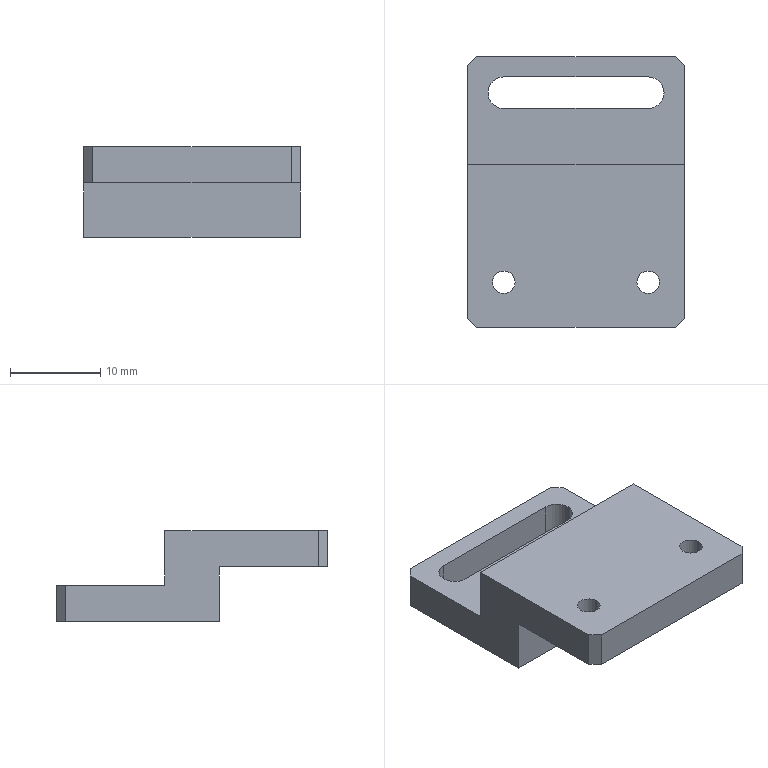Part | NX | features BREP 1 | 1 solid | 23 faces | box 24 x 30 x 10 mm | volume 3434 mm3 | plane 16 | cylinder 7 | commonest cylinder face diameters 2.5 x4 3.5 x3
STEP:
#1=CARTESIAN_POINT('',(9.25,-10.,6.));
#2=VERTEX_POINT('',#1);
#3=CARTESIAN_POINT('',(6.75,-10.,6.));
#4=VERTEX_POINT('',#3);
#5=CARTESIAN_POINT('',(8.,-10.,6.));
#6=DIRECTION('',(0.,0.,-1.));
#7=DIRECTION('',(1.,0.,0.));
#8=AXIS2_PLACEMENT_3D('',#5,#6,#7);
#9=CIRCLE('',#8,1.25);
#10=EDGE_CURVE('',#2,#4,#9,.T.);
#11=ORIENTED_EDGE('',*,*,#10,.T.);
#12=CARTESIAN_POINT('',(6.75,-10.,10.));
#13=VERTEX_POINT('',#12);
#14=CARTESIAN_POINT('',(6.75,-10.,10.));
#15=DIRECTION('',(0.,0.,1.));
#16=VECTOR('',#15,1000.);
#17=LINE('',#14,#16);
#18=EDGE_CURVE('',#13,#4,#17,.F.);
#19=ORIENTED_EDGE('',*,*,#18,.F.);
#20=CARTESIAN_POINT('',(9.25,-10.,10.));
#21=VERTEX_POINT('',#20);
#22=CARTESIAN_POINT('',(8.,-10.,10.));
#23=DIRECTION('',(0.,0.,1.));
#24=DIRECTION('',(1.,0.,0.));
#25=AXIS2_PLACEMENT_3D('',#22,#23,#24);
#26=CIRCLE('',#25,1.25);
#27=EDGE_CURVE('',#13,#21,#26,.T.);
#28=ORIENTED_EDGE('',*,*,#27,.T.);
#29=CARTESIAN_POINT('',(9.25,-10.,10.));
#30=DIRECTION('',(0.,0.,1.));
#31=VECTOR('',#30,1000.);
#32=LINE('',#29,#31);
#33=EDGE_CURVE('',#21,#2,#32,.F.);
#34=ORIENTED_EDGE('',*,*,#33,.T.);
#35=EDGE_LOOP('',(#11,#19,#28,#34));
#36=FACE_BOUND('',#35,.T.);
#37=CARTESIAN_POINT('',(8.,-10.,10.));
#38=DIRECTION('',(0.,0.,1.));
#39=DIRECTION('',(1.,0.,0.));
#40=AXIS2_PLACEMENT_3D('',#37,#38,#39);
#41=CYLINDRICAL_SURFACE('',#40,1.25);
#42=ADVANCED_FACE('',(#36),#41,.F.);
#43=CARTESIAN_POINT('',(-6.75,-10.,10.));
#44=VERTEX_POINT('',#43);
#45=CARTESIAN_POINT('',(-9.25,-10.,10.));
#46=VERTEX_POINT('',#45);
#47=CARTESIAN_POINT('',(-8.,-10.,10.));
#48=DIRECTION('',(0.,0.,-1.));
#49=DIRECTION('',(-1.,0.,0.));
#50=AXIS2_PLACEMENT_3D('',#47,#48,#49);
#51=CIRCLE('',#50,1.25);
#52=EDGE_CURVE('',#44,#46,#51,.T.);
#53=ORIENTED_EDGE('',*,*,#52,.F.);
#54=CARTESIAN_POINT('',(-6.75,-10.,6.));
#55=VERTEX_POINT('',#54);
#56=CARTESIAN_POINT('',(-6.75,-10.,0.));
#57=DIRECTION('',(0.,0.,-1.));
#58=VECTOR('',#57,1000.);
#59=LINE('',#56,#58);
#60=EDGE_CURVE('',#44,#55,#59,.T.);
#61=ORIENTED_EDGE('',*,*,#60,.T.);
#62=CARTESIAN_POINT('',(-9.25,-10.,6.));
#63=VERTEX_POINT('',#62);
#64=CARTESIAN_POINT('',(-8.,-10.,6.));
#65=DIRECTION('',(0.,0.,-1.));
#66=DIRECTION('',(1.,0.,0.));
#67=AXIS2_PLACEMENT_3D('',#64,#65,#66);
#68=CIRCLE('',#67,1.25);
#69=EDGE_CURVE('',#55,#63,#68,.T.);
#70=ORIENTED_EDGE('',*,*,#69,.T.);
#71=CARTESIAN_POINT('',(-9.25,-10.,0.));
#72=DIRECTION('',(0.,0.,-1.));
#73=VECTOR('',#72,1000.);
#74=LINE('',#71,#73);
#75=EDGE_CURVE('',#46,#63,#74,.T.);
#76=ORIENTED_EDGE('',*,*,#75,.F.);
#77=EDGE_LOOP('',(#53,#61,#70,#76));
#78=FACE_BOUND('',#77,.T.);
#79=CARTESIAN_POINT('',(-8.,-10.,0.));
#80=DIRECTION('',(0.,0.,-1.));
#81=DIRECTION('',(-1.,0.,0.));
#82=AXIS2_PLACEMENT_3D('',#79,#80,#81);
#83=CYLINDRICAL_SURFACE('',#82,1.25);
#84=ADVANCED_FACE('',(#78),#83,.F.);
#85=CARTESIAN_POINT('',(8.,12.75,0.));
#86=VERTEX_POINT('',#85);
#87=CARTESIAN_POINT('',(9.75,11.,0.));
#88=VERTEX_POINT('',#87);
#89=CARTESIAN_POINT('',(8.,11.,0.));
#90=DIRECTION('',(0.,0.,-1.));
#91=DIRECTION('',(-1.,0.,0.));
#92=AXIS2_PLACEMENT_3D('',#89,#90,#91);
#93=CIRCLE('',#92,1.75);
#94=EDGE_CURVE('',#86,#88,#93,.T.);
#95=ORIENTED_EDGE('',*,*,#94,.T.);
#96=CARTESIAN_POINT('',(9.75,11.,4.));
#97=VERTEX_POINT('',#96);
#98=CARTESIAN_POINT('',(9.75,11.,-5.));
#99=DIRECTION('',(0.,0.,1.));
#100=VECTOR('',#99,1000.);
#101=LINE('',#98,#100);
#102=EDGE_CURVE('',#88,#97,#101,.T.);
#103=ORIENTED_EDGE('',*,*,#102,.T.);
#104=CARTESIAN_POINT('',(8.,12.75,4.));
#105=VERTEX_POINT('',#104);
#106=CARTESIAN_POINT('',(8.,11.,4.));
#107=DIRECTION('',(0.,0.,1.));
#108=DIRECTION('',(-1.,0.,0.));
#109=AXIS2_PLACEMENT_3D('',#106,#107,#108);
#110=CIRCLE('',#109,1.75);
#111=EDGE_CURVE('',#97,#105,#110,.T.);
#112=ORIENTED_EDGE('',*,*,#111,.T.);
#113=CARTESIAN_POINT('',(8.,12.75,-5.));
#114=DIRECTION('',(0.,0.,1.));
#115=VECTOR('',#114,1000.);
#116=LINE('',#113,#115);
#117=EDGE_CURVE('',#86,#105,#116,.T.);
#118=ORIENTED_EDGE('',*,*,#117,.F.);
#119=EDGE_LOOP('',(#95,#103,#112,#118));
#120=FACE_BOUND('',#119,.T.);
#121=CARTESIAN_POINT('',(8.,11.,-5.));
#122=DIRECTION('',(0.,0.,1.));
#123=DIRECTION('',(1.,0.,0.));
#124=AXIS2_PLACEMENT_3D('',#121,#122,#123);
#125=CYLINDRICAL_SURFACE('',#124,1.75);
#126=ADVANCED_FACE('',(#120),#125,.F.);
#127=CARTESIAN_POINT('',(12.,-3.,0.));
#128=VERTEX_POINT('',#127);
#129=CARTESIAN_POINT('',(12.,14.,0.));
#130=VERTEX_POINT('',#129);
#131=CARTESIAN_POINT('',(12.,-15.,0.));
#132=DIRECTION('',(0.,1.,0.));
#133=VECTOR('',#132,1000.);
#134=LINE('',#131,#133);
#135=EDGE_CURVE('',#128,#130,#134,.T.);
#136=ORIENTED_EDGE('',*,*,#135,.T.);
#137=CARTESIAN_POINT('',(12.,14.,4.));
#138=VERTEX_POINT('',#137);
#139=CARTESIAN_POINT('',(12.,14.,10.));
#140=DIRECTION('',(0.,0.,1.));
#141=VECTOR('',#140,1000.);
#142=LINE('',#139,#141);
#143=EDGE_CURVE('',#130,#138,#142,.T.);
#144=ORIENTED_EDGE('',*,*,#143,.T.);
#145=CARTESIAN_POINT('',(12.,3.,4.));
#146=VERTEX_POINT('',#145);
#147=CARTESIAN_POINT('',(12.,3.,4.));
#148=DIRECTION('',(0.,1.,0.));
#149=VECTOR('',#148,1000.);
#150=LINE('',#147,#149);
#151=EDGE_CURVE('',#146,#138,#150,.T.);
#152=ORIENTED_EDGE('',*,*,#151,.F.);
#153=CARTESIAN_POINT('',(12.,3.,10.));
#154=VERTEX_POINT('',#153);
#155=CARTESIAN_POINT('',(12.,3.,10.));
#156=DIRECTION('',(0.,0.,-1.));
#157=VECTOR('',#156,1000.);
#158=LINE('',#155,#157);
#159=EDGE_CURVE('',#154,#146,#158,.T.);
#160=ORIENTED_EDGE('',*,*,#159,.F.);
#161=CARTESIAN_POINT('',(12.,-14.,10.));
#162=VERTEX_POINT('',#161);
#163=CARTESIAN_POINT('',(12.,-15.,10.));
#164=DIRECTION('',(0.,1.,0.));
#165=VECTOR('',#164,1000.);
#166=LINE('',#163,#165);
#167=EDGE_CURVE('',#162,#154,#166,.T.);
#168=ORIENTED_EDGE('',*,*,#167,.F.);
#169=CARTESIAN_POINT('',(12.,-14.,6.));
#170=VERTEX_POINT('',#169);
#171=CARTESIAN_POINT('',(12.,-14.,10.));
#172=DIRECTION('',(0.,0.,-1.));
#173=VECTOR('',#172,1000.);
#174=LINE('',#171,#173);
#175=EDGE_CURVE('',#162,#170,#174,.T.);
#176=ORIENTED_EDGE('',*,*,#175,.T.);
#177=CARTESIAN_POINT('',(12.,-3.,6.));
#178=VERTEX_POINT('',#177);
#179=CARTESIAN_POINT('',(12.,-15.,6.));
#180=DIRECTION('',(0.,1.,0.));
#181=VECTOR('',#180,1000.);
#182=LINE('',#179,#181);
#183=EDGE_CURVE('',#170,#178,#182,.T.);
#184=ORIENTED_EDGE('',*,*,#183,.T.);
#185=CARTESIAN_POINT('',(12.,-3.,10.));
#186=DIRECTION('',(0.,0.,-1.));
#187=VECTOR('',#186,1000.);
#188=LINE('',#185,#187);
#189=EDGE_CURVE('',#178,#128,#188,.T.);
#190=ORIENTED_EDGE('',*,*,#189,.T.);
#191=EDGE_LOOP('',(#136,#144,#152,#160,#168,#176,#184,#190));
#192=FACE_BOUND('',#191,.T.);
#193=CARTESIAN_POINT('',(12.,-15.,10.));
#194=DIRECTION('',(-1.,0.,0.));
#195=DIRECTION('',(0.,0.,1.));
#196=AXIS2_PLACEMENT_3D('',#193,#194,#195);
#197=PLANE('',#196);
#198=ADVANCED_FACE('',(#192),#197,.F.);
#199=CARTESIAN_POINT('',(-11.,15.,4.));
#200=VERTEX_POINT('',#199);
#201=CARTESIAN_POINT('',(11.,15.,4.));
#202=VERTEX_POINT('',#201);
#203=CARTESIAN_POINT('',(-18.,15.,4.));
#204=DIRECTION('',(1.,0.,0.));
#205=VECTOR('',#204,1000.);
#206=LINE('',#203,#205);
#207=EDGE_CURVE('',#200,#202,#206,.T.);
#208=ORIENTED_EDGE('',*,*,#207,.T.);
#209=CARTESIAN_POINT('',(11.,15.,0.));
#210=VERTEX_POINT('',#209);
#211=CARTESIAN_POINT('',(11.,15.,10.));
#212=DIRECTION('',(0.,0.,-1.));
#213=VECTOR('',#212,1000.);
#214=LINE('',#211,#213);
#215=EDGE_CURVE('',#202,#210,#214,.T.);
#216=ORIENTED_EDGE('',*,*,#215,.T.);
#217=CARTESIAN_POINT('',(-11.,15.,0.));
#218=VERTEX_POINT('',#217);
#219=CARTESIAN_POINT('',(-12.,15.,0.));
#220=DIRECTION('',(-1.,0.,0.));
#221=VECTOR('',#220,1000.);
#222=LINE('',#219,#221);
#223=EDGE_CURVE('',#210,#218,#222,.T.);
#224=ORIENTED_EDGE('',*,*,#223,.T.);
#225=CARTESIAN_POINT('',(-11.,15.,10.));
#226=DIRECTION('',(0.,0.,1.));
#227=VECTOR('',#226,1000.);
#228=LINE('',#225,#227);
#229=EDGE_CURVE('',#218,#200,#228,.T.);
#230=ORIENTED_EDGE('',*,*,#229,.T.);
#231=EDGE_LOOP('',(#208,#216,#224,#230));
#232=FACE_BOUND('',#231,.T.);
#233=CARTESIAN_POINT('',(-12.,15.,10.));
#234=DIRECTION('',(0.,-1.,0.));
#235=DIRECTION('',(0.,0.,-1.));
#236=AXIS2_PLACEMENT_3D('',#233,#234,#235);
#237=PLANE('',#236);
#238=ADVANCED_FACE('',(#232),#237,.F.);
#239=CARTESIAN_POINT('',(-12.,3.,4.));
#240=VERTEX_POINT('',#239);
#241=CARTESIAN_POINT('',(-12.,14.,4.));
#242=VERTEX_POINT('',#241);
#243=CARTESIAN_POINT('',(-12.,-15.,4.));
#244=DIRECTION('',(0.,1.,0.));
#245=VECTOR('',#244,1000.);
#246=LINE('',#243,#245);
#247=EDGE_CURVE('',#240,#242,#246,.T.);
#248=ORIENTED_EDGE('',*,*,#247,.T.);
#249=CARTESIAN_POINT('',(-12.,14.,0.));
#250=VERTEX_POINT('',#249);
#251=CARTESIAN_POINT('',(-12.,14.,10.));
#252=DIRECTION('',(0.,0.,-1.));
#253=VECTOR('',#252,1000.);
#254=LINE('',#251,#253);
#255=EDGE_CURVE('',#242,#250,#254,.T.);
#256=ORIENTED_EDGE('',*,*,#255,.T.);
#257=CARTESIAN_POINT('',(-12.,-3.,0.));
#258=VERTEX_POINT('',#257);
#259=CARTESIAN_POINT('',(-12.,-15.,0.));
#260=DIRECTION('',(0.,-1.,0.));
#261=VECTOR('',#260,1000.);
#262=LINE('',#259,#261);
#263=EDGE_CURVE('',#250,#258,#262,.T.);
#264=ORIENTED_EDGE('',*,*,#263,.T.);
#265=CARTESIAN_POINT('',(-12.,-3.,6.));
#266=VERTEX_POINT('',#265);
#267=CARTESIAN_POINT('',(-12.,-3.,6.));
#268=DIRECTION('',(0.,0.,-1.));
#269=VECTOR('',#268,1000.);
#270=LINE('',#267,#269);
#271=EDGE_CURVE('',#266,#258,#270,.T.);
#272=ORIENTED_EDGE('',*,*,#271,.F.);
#273=CARTESIAN_POINT('',(-12.,-14.,6.));
#274=VERTEX_POINT('',#273);
#275=CARTESIAN_POINT('',(-12.,-15.,6.));
#276=DIRECTION('',(0.,1.,0.));
#277=VECTOR('',#276,1000.);
#278=LINE('',#275,#277);
#279=EDGE_CURVE('',#274,#266,#278,.T.);
#280=ORIENTED_EDGE('',*,*,#279,.F.);
#281=CARTESIAN_POINT('',(-12.,-14.,10.));
#282=VERTEX_POINT('',#281);
#283=CARTESIAN_POINT('',(-12.,-14.,10.));
#284=DIRECTION('',(0.,0.,1.));
#285=VECTOR('',#284,1000.);
#286=LINE('',#283,#285);
#287=EDGE_CURVE('',#274,#282,#286,.T.);
#288=ORIENTED_EDGE('',*,*,#287,.T.);
#289=CARTESIAN_POINT('',(-12.,3.,10.));
#290=VERTEX_POINT('',#289);
#291=CARTESIAN_POINT('',(-12.,-15.,10.));
#292=DIRECTION('',(0.,-1.,0.));
#293=VECTOR('',#292,1000.);
#294=LINE('',#291,#293);
#295=EDGE_CURVE('',#290,#282,#294,.T.);
#296=ORIENTED_EDGE('',*,*,#295,.F.);
#297=CARTESIAN_POINT('',(-12.,3.,10.));
#298=DIRECTION('',(0.,0.,-1.));
#299=VECTOR('',#298,1000.);
#300=LINE('',#297,#299);
#301=EDGE_CURVE('',#290,#240,#300,.T.);
#302=ORIENTED_EDGE('',*,*,#301,.T.);
#303=EDGE_LOOP('',(#248,#256,#264,#272,#280,#288,#296,#302));
#304=FACE_BOUND('',#303,.T.);
#305=CARTESIAN_POINT('',(-12.,-15.,10.));
#306=DIRECTION('',(1.,0.,0.));
#307=DIRECTION('',(0.,1.,0.));
#308=AXIS2_PLACEMENT_3D('',#305,#306,#307);
#309=PLANE('',#308);
#310=ADVANCED_FACE('',(#304),#309,.F.);
#311=CARTESIAN_POINT('',(-11.,-15.,10.));
#312=VERTEX_POINT('',#311);
#313=CARTESIAN_POINT('',(11.,-15.,10.));
#314=VERTEX_POINT('',#313);
#315=CARTESIAN_POINT('',(-12.,-15.,10.));
#316=DIRECTION('',(1.,0.,0.));
#317=VECTOR('',#316,1000.);
#318=LINE('',#315,#317);
#319=EDGE_CURVE('',#312,#314,#318,.T.);
#320=ORIENTED_EDGE('',*,*,#319,.F.);
#321=CARTESIAN_POINT('',(-11.,-15.,6.));
#322=VERTEX_POINT('',#321);
#323=CARTESIAN_POINT('',(-11.,-15.,10.));
#324=DIRECTION('',(0.,0.,-1.));
#325=VECTOR('',#324,1000.);
#326=LINE('',#323,#325);
#327=EDGE_CURVE('',#312,#322,#326,.T.);
#328=ORIENTED_EDGE('',*,*,#327,.T.);
#329=CARTESIAN_POINT('',(11.,-15.,6.));
#330=VERTEX_POINT('',#329);
#331=CARTESIAN_POINT('',(18.,-15.,6.));
#332=DIRECTION('',(-1.,0.,0.));
#333=VECTOR('',#332,1000.);
#334=LINE('',#331,#333);
#335=EDGE_CURVE('',#330,#322,#334,.T.);
#336=ORIENTED_EDGE('',*,*,#335,.F.);
#337=CARTESIAN_POINT('',(11.,-15.,10.));
#338=DIRECTION('',(0.,0.,1.));
#339=VECTOR('',#338,1000.);
#340=LINE('',#337,#339);
#341=EDGE_CURVE('',#330,#314,#340,.T.);
#342=ORIENTED_EDGE('',*,*,#341,.T.);
#343=EDGE_LOOP('',(#320,#328,#336,#342));
#344=FACE_BOUND('',#343,.T.);
#345=CARTESIAN_POINT('',(-12.,-15.,10.));
#346=DIRECTION('',(0.,1.,0.));
#347=DIRECTION('',(1.,0.,0.));
#348=AXIS2_PLACEMENT_3D('',#345,#346,#347);
#349=PLANE('',#348);
#350=ADVANCED_FACE('',(#344),#349,.F.);
#351=ORIENTED_EDGE('',*,*,#295,.T.);
#352=CARTESIAN_POINT('',(-11.,-15.,10.));
#353=DIRECTION('',(0.7071,-0.7071,0.));
#354=VECTOR('',#353,1000.);
#355=LINE('',#352,#354);
#356=EDGE_CURVE('',#282,#312,#355,.T.);
#357=ORIENTED_EDGE('',*,*,#356,.T.);
#358=ORIENTED_EDGE('',*,*,#319,.T.);
#359=CARTESIAN_POINT('',(12.,-14.,10.));
#360=DIRECTION('',(0.7071,0.7071,0.));
#361=VECTOR('',#360,1000.);
#362=LINE('',#359,#361);
#363=EDGE_CURVE('',#314,#162,#362,.T.);
#364=ORIENTED_EDGE('',*,*,#363,.T.);
#365=ORIENTED_EDGE('',*,*,#167,.T.);
#366=CARTESIAN_POINT('',(-18.,3.,10.));
#367=DIRECTION('',(1.,0.,0.));
#368=VECTOR('',#367,1000.);
#369=LINE('',#366,#368);
#370=EDGE_CURVE('',#290,#154,#369,.T.);
#371=ORIENTED_EDGE('',*,*,#370,.F.);
#372=EDGE_LOOP('',(#351,#357,#358,#364,#365,#371));
#373=FACE_BOUND('',#372,.T.);
#374=CARTESIAN_POINT('',(8.,-10.,10.));
#375=DIRECTION('',(0.,0.,1.));
#376=DIRECTION('',(1.,0.,0.));
#377=AXIS2_PLACEMENT_3D('',#374,#375,#376);
#378=CIRCLE('',#377,1.25);
#379=EDGE_CURVE('',#21,#13,#378,.T.);
#380=ORIENTED_EDGE('',*,*,#379,.F.);
#381=ORIENTED_EDGE('',*,*,#27,.F.);
#382=EDGE_LOOP('',(#380,#381));
#383=FACE_BOUND('',#382,.T.);
#384=CARTESIAN_POINT('',(-8.,-10.,10.));
#385=DIRECTION('',(0.,0.,-1.));
#386=DIRECTION('',(-1.,0.,0.));
#387=AXIS2_PLACEMENT_3D('',#384,#385,#386);
#388=CIRCLE('',#387,1.25);
#389=EDGE_CURVE('',#46,#44,#388,.T.);
#390=ORIENTED_EDGE('',*,*,#389,.T.);
#391=ORIENTED_EDGE('',*,*,#52,.T.);
#392=EDGE_LOOP('',(#390,#391));
#393=FACE_BOUND('',#392,.T.);
#394=CARTESIAN_POINT('',(12.,15.,10.));
#395=DIRECTION('',(0.,0.,-1.));
#396=DIRECTION('',(0.,-1.,0.));
#397=AXIS2_PLACEMENT_3D('',#394,#395,#396);
#398=PLANE('',#397);
#399=ADVANCED_FACE('',(#373,#383,#393),#398,.F.);
#400=ORIENTED_EDGE('',*,*,#223,.F.);
#401=CARTESIAN_POINT('',(11.5,14.5,0.));
#402=DIRECTION('',(0.7071,-0.7071,0.));
#403=VECTOR('',#402,1000.);
#404=LINE('',#401,#403);
#405=EDGE_CURVE('',#210,#130,#404,.T.);
#406=ORIENTED_EDGE('',*,*,#405,.T.);
#407=ORIENTED_EDGE('',*,*,#135,.F.);
#408=CARTESIAN_POINT('',(18.,-3.,0.));
#409=DIRECTION('',(-1.,0.,0.));
#410=VECTOR('',#409,1000.);
#411=LINE('',#408,#410);
#412=EDGE_CURVE('',#128,#258,#411,.T.);
#413=ORIENTED_EDGE('',*,*,#412,.T.);
#414=ORIENTED_EDGE('',*,*,#263,.F.);
#415=CARTESIAN_POINT('',(0.5,26.5,0.));
#416=DIRECTION('',(0.7071,0.7071,0.));
#417=VECTOR('',#416,1000.);
#418=LINE('',#415,#417);
#419=EDGE_CURVE('',#250,#218,#418,.T.);
#420=ORIENTED_EDGE('',*,*,#419,.T.);
#421=EDGE_LOOP('',(#400,#406,#407,#413,#414,#420));
#422=FACE_BOUND('',#421,.T.);
#423=CARTESIAN_POINT('',(-8.,9.25,0.));
#424=VERTEX_POINT('',#423);
#425=CARTESIAN_POINT('',(-8.,12.75,0.));
#426=VERTEX_POINT('',#425);
#427=CARTESIAN_POINT('',(-8.,11.,0.));
#428=DIRECTION('',(0.,0.,-1.));
#429=DIRECTION('',(-1.,0.,0.));
#430=AXIS2_PLACEMENT_3D('',#427,#428,#429);
#431=CIRCLE('',#430,1.75);
#432=EDGE_CURVE('',#424,#426,#431,.T.);
#433=ORIENTED_EDGE('',*,*,#432,.F.);
#434=CARTESIAN_POINT('',(8.,9.25,0.));
#435=VERTEX_POINT('',#434);
#436=CARTESIAN_POINT('',(12.,9.25,0.));
#437=DIRECTION('',(-1.,0.,0.));
#438=VECTOR('',#437,1000.);
#439=LINE('',#436,#438);
#440=EDGE_CURVE('',#435,#424,#439,.T.);
#441=ORIENTED_EDGE('',*,*,#440,.F.);
#442=CARTESIAN_POINT('',(8.,11.,0.));
#443=DIRECTION('',(0.,0.,-1.));
#444=DIRECTION('',(-1.,0.,0.));
#445=AXIS2_PLACEMENT_3D('',#442,#443,#444);
#446=CIRCLE('',#445,1.75);
#447=EDGE_CURVE('',#88,#435,#446,.T.);
#448=ORIENTED_EDGE('',*,*,#447,.F.);
#449=ORIENTED_EDGE('',*,*,#94,.F.);
#450=CARTESIAN_POINT('',(12.,12.75,0.));
#451=DIRECTION('',(1.,0.,0.));
#452=VECTOR('',#451,1000.);
#453=LINE('',#450,#452);
#454=EDGE_CURVE('',#426,#86,#453,.T.);
#455=ORIENTED_EDGE('',*,*,#454,.F.);
#456=EDGE_LOOP('',(#433,#441,#448,#449,#455));
#457=FACE_BOUND('',#456,.T.);
#458=CARTESIAN_POINT('',(12.,15.,0.));
#459=DIRECTION('',(0.,0.,-1.));
#460=DIRECTION('',(0.,-1.,0.));
#461=AXIS2_PLACEMENT_3D('',#458,#459,#460);
#462=PLANE('',#461);
#463=ADVANCED_FACE('',(#422,#457),#462,.T.);
#464=CARTESIAN_POINT('',(-8.,12.75,4.));
#465=VERTEX_POINT('',#464);
#466=CARTESIAN_POINT('',(-8.,12.75,-5.));
#467=DIRECTION('',(0.,0.,1.));
#468=VECTOR('',#467,1000.);
#469=LINE('',#466,#468);
#470=EDGE_CURVE('',#426,#465,#469,.T.);
#471=ORIENTED_EDGE('',*,*,#470,.T.);
#472=CARTESIAN_POINT('',(-8.,9.25,4.));
#473=VERTEX_POINT('',#472);
#474=CARTESIAN_POINT('',(-8.,11.,4.));
#475=DIRECTION('',(0.,0.,1.));
#476=DIRECTION('',(-1.,0.,0.));
#477=AXIS2_PLACEMENT_3D('',#474,#475,#476);
#478=CIRCLE('',#477,1.75);
#479=EDGE_CURVE('',#465,#473,#478,.T.);
#480=ORIENTED_EDGE('',*,*,#479,.T.);
#481=CARTESIAN_POINT('',(-8.,9.25,-5.));
#482=DIRECTION('',(0.,0.,1.));
#483=VECTOR('',#482,1000.);
#484=LINE('',#481,#483);
#485=EDGE_CURVE('',#424,#473,#484,.T.);
#486=ORIENTED_EDGE('',*,*,#485,.F.);
#487=ORIENTED_EDGE('',*,*,#432,.T.);
#488=EDGE_LOOP('',(#471,#480,#486,#487));
#489=FACE_BOUND('',#488,.T.);
#490=CARTESIAN_POINT('',(-8.,11.,-5.));
#491=DIRECTION('',(0.,0.,1.));
#492=DIRECTION('',(1.,0.,0.));
#493=AXIS2_PLACEMENT_3D('',#490,#491,#492);
#494=CYLINDRICAL_SURFACE('',#493,1.75);
#495=ADVANCED_FACE('',(#489),#494,.F.);
#496=ORIENTED_EDGE('',*,*,#117,.T.);
#497=CARTESIAN_POINT('',(-8.,12.75,4.));
#498=DIRECTION('',(-1.,0.,0.));
#499=VECTOR('',#498,1000.);
#500=LINE('',#497,#499);
#501=EDGE_CURVE('',#105,#465,#500,.T.);
#502=ORIENTED_EDGE('',*,*,#501,.T.);
#503=ORIENTED_EDGE('',*,*,#470,.F.);
#504=ORIENTED_EDGE('',*,*,#454,.T.);
#505=EDGE_LOOP('',(#496,#502,#503,#504));
#506=FACE_BOUND('',#505,.T.);
#507=CARTESIAN_POINT('',(-8.,12.75,-5.));
#508=DIRECTION('',(0.,1.,0.));
#509=DIRECTION('',(1.,0.,0.));
#510=AXIS2_PLACEMENT_3D('',#507,#508,#509);
#511=PLANE('',#510);
#512=ADVANCED_FACE('',(#506),#511,.F.);
#513=ORIENTED_EDGE('',*,*,#102,.F.);
#514=ORIENTED_EDGE('',*,*,#447,.T.);
#515=CARTESIAN_POINT('',(8.,9.25,4.));
#516=VERTEX_POINT('',#515);
#517=CARTESIAN_POINT('',(8.,9.25,-5.));
#518=DIRECTION('',(0.,0.,1.));
#519=VECTOR('',#518,1000.);
#520=LINE('',#517,#519);
#521=EDGE_CURVE('',#435,#516,#520,.T.);
#522=ORIENTED_EDGE('',*,*,#521,.T.);
#523=CARTESIAN_POINT('',(8.,11.,4.));
#524=DIRECTION('',(0.,0.,1.));
#525=DIRECTION('',(-1.,0.,0.));
#526=AXIS2_PLACEMENT_3D('',#523,#524,#525);
#527=CIRCLE('',#526,1.75);
#528=EDGE_CURVE('',#516,#97,#527,.T.);
#529=ORIENTED_EDGE('',*,*,#528,.T.);
#530=EDGE_LOOP('',(#513,#514,#522,#529));
#531=FACE_BOUND('',#530,.T.);
#532=CARTESIAN_POINT('',(8.,11.,-5.));
#533=DIRECTION('',(0.,0.,1.));
#534=DIRECTION('',(1.,0.,0.));
#535=AXIS2_PLACEMENT_3D('',#532,#533,#534);
#536=CYLINDRICAL_SURFACE('',#535,1.75);
#537=ADVANCED_FACE('',(#531),#536,.F.);
#538=ORIENTED_EDGE('',*,*,#485,.T.);
#539=CARTESIAN_POINT('',(-8.,9.25,4.));
#540=DIRECTION('',(1.,0.,0.));
#541=VECTOR('',#540,1000.);
#542=LINE('',#539,#541);
#543=EDGE_CURVE('',#473,#516,#542,.T.);
#544=ORIENTED_EDGE('',*,*,#543,.T.);
#545=ORIENTED_EDGE('',*,*,#521,.F.);
#546=ORIENTED_EDGE('',*,*,#440,.T.);
#547=EDGE_LOOP('',(#538,#544,#545,#546));
#548=FACE_BOUND('',#547,.T.);
#549=CARTESIAN_POINT('',(-8.,9.25,-5.));
#550=DIRECTION('',(0.,-1.,0.));
#551=DIRECTION('',(0.,0.,-1.));
#552=AXIS2_PLACEMENT_3D('',#549,#550,#551);
#553=PLANE('',#552);
#554=ADVANCED_FACE('',(#548),#553,.F.);
#555=ORIENTED_EDGE('',*,*,#60,.F.);
#556=ORIENTED_EDGE('',*,*,#389,.F.);
#557=ORIENTED_EDGE('',*,*,#75,.T.);
#558=CARTESIAN_POINT('',(-8.,-10.,6.));
#559=DIRECTION('',(0.,0.,-1.));
#560=DIRECTION('',(1.,0.,0.));
#561=AXIS2_PLACEMENT_3D('',#558,#559,#560);
#562=CIRCLE('',#561,1.25);
#563=EDGE_CURVE('',#63,#55,#562,.T.);
#564=ORIENTED_EDGE('',*,*,#563,.T.);
#565=EDGE_LOOP('',(#555,#556,#557,#564));
#566=FACE_BOUND('',#565,.T.);
#567=CARTESIAN_POINT('',(-8.,-10.,0.));
#568=DIRECTION('',(0.,0.,-1.));
#569=DIRECTION('',(-1.,0.,0.));
#570=AXIS2_PLACEMENT_3D('',#567,#568,#569);
#571=CYLINDRICAL_SURFACE('',#570,1.25);
#572=ADVANCED_FACE('',(#566),#571,.F.);
#573=ORIENTED_EDGE('',*,*,#18,.T.);
#574=CARTESIAN_POINT('',(8.,-10.,6.));
#575=DIRECTION('',(0.,0.,-1.));
#576=DIRECTION('',(1.,0.,0.));
#577=AXIS2_PLACEMENT_3D('',#574,#575,#576);
#578=CIRCLE('',#577,1.25);
#579=EDGE_CURVE('',#4,#2,#578,.T.);
#580=ORIENTED_EDGE('',*,*,#579,.T.);
#581=ORIENTED_EDGE('',*,*,#33,.F.);
#582=ORIENTED_EDGE('',*,*,#379,.T.);
#583=EDGE_LOOP('',(#573,#580,#581,#582));
#584=FACE_BOUND('',#583,.T.);
#585=CARTESIAN_POINT('',(8.,-10.,10.));
#586=DIRECTION('',(0.,0.,1.));
#587=DIRECTION('',(1.,0.,0.));
#588=AXIS2_PLACEMENT_3D('',#585,#586,#587);
#589=CYLINDRICAL_SURFACE('',#588,1.25);
#590=ADVANCED_FACE('',(#584),#589,.F.);
#591=CARTESIAN_POINT('',(18.,-3.,6.));
#592=DIRECTION('',(-1.,0.,0.));
#593=VECTOR('',#592,1000.);
#594=LINE('',#591,#593);
#595=EDGE_CURVE('',#178,#266,#594,.T.);
#596=ORIENTED_EDGE('',*,*,#595,.T.);
#597=ORIENTED_EDGE('',*,*,#271,.T.);
#598=ORIENTED_EDGE('',*,*,#412,.F.);
#599=ORIENTED_EDGE('',*,*,#189,.F.);
#600=EDGE_LOOP('',(#596,#597,#598,#599));
#601=FACE_BOUND('',#600,.T.);
#602=CARTESIAN_POINT('',(18.,-3.,6.));
#603=DIRECTION('',(0.,1.,0.));
#604=DIRECTION('',(1.,0.,0.));
#605=AXIS2_PLACEMENT_3D('',#602,#603,#604);
#606=PLANE('',#605);
#607=ADVANCED_FACE('',(#601),#606,.F.);
#608=ORIENTED_EDGE('',*,*,#335,.T.);
#609=CARTESIAN_POINT('',(-11.,-15.,6.));
#610=DIRECTION('',(-0.7071,0.7071,0.));
#611=VECTOR('',#610,1000.);
#612=LINE('',#609,#611);
#613=EDGE_CURVE('',#322,#274,#612,.T.);
#614=ORIENTED_EDGE('',*,*,#613,.T.);
#615=ORIENTED_EDGE('',*,*,#279,.T.);
#616=ORIENTED_EDGE('',*,*,#595,.F.);
#617=ORIENTED_EDGE('',*,*,#183,.F.);
#618=CARTESIAN_POINT('',(12.,-14.,6.));
#619=DIRECTION('',(-0.7071,-0.7071,0.));
#620=VECTOR('',#619,1000.);
#621=LINE('',#618,#620);
#622=EDGE_CURVE('',#170,#330,#621,.T.);
#623=ORIENTED_EDGE('',*,*,#622,.T.);
#624=EDGE_LOOP('',(#608,#614,#615,#616,#617,#623));
#625=FACE_BOUND('',#624,.T.);
#626=ORIENTED_EDGE('',*,*,#563,.F.);
#627=ORIENTED_EDGE('',*,*,#69,.F.);
#628=EDGE_LOOP('',(#626,#627));
#629=FACE_BOUND('',#628,.T.);
#630=ORIENTED_EDGE('',*,*,#10,.F.);
#631=ORIENTED_EDGE('',*,*,#579,.F.);
#632=EDGE_LOOP('',(#630,#631));
#633=FACE_BOUND('',#632,.T.);
#634=CARTESIAN_POINT('',(18.,-15.,6.));
#635=DIRECTION('',(0.,0.,1.));
#636=DIRECTION('',(1.,0.,0.));
#637=AXIS2_PLACEMENT_3D('',#634,#635,#636);
#638=PLANE('',#637);
#639=ADVANCED_FACE('',(#625,#629,#633),#638,.F.);
#640=ORIENTED_EDGE('',*,*,#370,.T.);
#641=ORIENTED_EDGE('',*,*,#159,.T.);
#642=CARTESIAN_POINT('',(-18.,3.,4.));
#643=DIRECTION('',(1.,0.,0.));
#644=VECTOR('',#643,1000.);
#645=LINE('',#642,#644);
#646=EDGE_CURVE('',#240,#146,#645,.T.);
#647=ORIENTED_EDGE('',*,*,#646,.F.);
#648=ORIENTED_EDGE('',*,*,#301,.F.);
#649=EDGE_LOOP('',(#640,#641,#647,#648));
#650=FACE_BOUND('',#649,.T.);
#651=CARTESIAN_POINT('',(-18.,3.,10.));
#652=DIRECTION('',(0.,-1.,0.));
#653=DIRECTION('',(0.,0.,-1.));
#654=AXIS2_PLACEMENT_3D('',#651,#652,#653);
#655=PLANE('',#654);
#656=ADVANCED_FACE('',(#650),#655,.F.);
#657=ORIENTED_EDGE('',*,*,#151,.T.);
#658=CARTESIAN_POINT('',(11.,15.,4.));
#659=DIRECTION('',(-0.7071,0.7071,0.));
#660=VECTOR('',#659,1000.);
#661=LINE('',#658,#660);
#662=EDGE_CURVE('',#138,#202,#661,.T.);
#663=ORIENTED_EDGE('',*,*,#662,.T.);
#664=ORIENTED_EDGE('',*,*,#207,.F.);
#665=CARTESIAN_POINT('',(-12.,14.,4.));
#666=DIRECTION('',(-0.7071,-0.7071,0.));
#667=VECTOR('',#666,1000.);
#668=LINE('',#665,#667);
#669=EDGE_CURVE('',#200,#242,#668,.T.);
#670=ORIENTED_EDGE('',*,*,#669,.T.);
#671=ORIENTED_EDGE('',*,*,#247,.F.);
#672=ORIENTED_EDGE('',*,*,#646,.T.);
#673=EDGE_LOOP('',(#657,#663,#664,#670,#671,#672));
#674=FACE_BOUND('',#673,.T.);
#675=ORIENTED_EDGE('',*,*,#501,.F.);
#676=ORIENTED_EDGE('',*,*,#111,.F.);
#677=ORIENTED_EDGE('',*,*,#528,.F.);
#678=ORIENTED_EDGE('',*,*,#543,.F.);
#679=ORIENTED_EDGE('',*,*,#479,.F.);
#680=EDGE_LOOP('',(#675,#676,#677,#678,#679));
#681=FACE_BOUND('',#680,.T.);
#682=CARTESIAN_POINT('',(-18.,3.,4.));
#683=DIRECTION('',(0.,0.,-1.));
#684=DIRECTION('',(0.,-1.,0.));
#685=AXIS2_PLACEMENT_3D('',#682,#683,#684);
#686=PLANE('',#685);
#687=ADVANCED_FACE('',(#674,#681),#686,.F.);
#688=ORIENTED_EDGE('',*,*,#662,.F.);
#689=ORIENTED_EDGE('',*,*,#143,.F.);
#690=ORIENTED_EDGE('',*,*,#405,.F.);
#691=ORIENTED_EDGE('',*,*,#215,.F.);
#692=EDGE_LOOP('',(#688,#689,#690,#691));
#693=FACE_BOUND('',#692,.T.);
#694=CARTESIAN_POINT('',(11.,15.,10.));
#695=DIRECTION('',(-0.7071,-0.7071,0.));
#696=DIRECTION('',(-0.7071,0.7071,0.));
#697=AXIS2_PLACEMENT_3D('',#694,#695,#696);
#698=PLANE('',#697);
#699=ADVANCED_FACE('',(#693),#698,.F.);
#700=ORIENTED_EDGE('',*,*,#669,.F.);
#701=ORIENTED_EDGE('',*,*,#229,.F.);
#702=ORIENTED_EDGE('',*,*,#419,.F.);
#703=ORIENTED_EDGE('',*,*,#255,.F.);
#704=EDGE_LOOP('',(#700,#701,#702,#703));
#705=FACE_BOUND('',#704,.T.);
#706=CARTESIAN_POINT('',(-12.,14.,10.));
#707=DIRECTION('',(0.7071,-0.7071,0.));
#708=DIRECTION('',(0.,0.,-1.));
#709=AXIS2_PLACEMENT_3D('',#706,#707,#708);
#710=PLANE('',#709);
#711=ADVANCED_FACE('',(#705),#710,.F.);
#712=ORIENTED_EDGE('',*,*,#356,.F.);
#713=ORIENTED_EDGE('',*,*,#287,.F.);
#714=ORIENTED_EDGE('',*,*,#613,.F.);
#715=ORIENTED_EDGE('',*,*,#327,.F.);
#716=EDGE_LOOP('',(#712,#713,#714,#715));
#717=FACE_BOUND('',#716,.T.);
#718=CARTESIAN_POINT('',(-11.,-15.,10.));
#719=DIRECTION('',(0.7071,0.7071,0.));
#720=DIRECTION('',(0.,0.,-1.));
#721=AXIS2_PLACEMENT_3D('',#718,#719,#720);
#722=PLANE('',#721);
#723=ADVANCED_FACE('',(#717),#722,.F.);
#724=ORIENTED_EDGE('',*,*,#363,.F.);
#725=ORIENTED_EDGE('',*,*,#341,.F.);
#726=ORIENTED_EDGE('',*,*,#622,.F.);
#727=ORIENTED_EDGE('',*,*,#175,.F.);
#728=EDGE_LOOP('',(#724,#725,#726,#727));
#729=FACE_BOUND('',#728,.T.);
#730=CARTESIAN_POINT('',(12.,-14.,10.));
#731=DIRECTION('',(-0.7071,0.7071,0.));
#732=DIRECTION('',(0.,0.,1.));
#733=AXIS2_PLACEMENT_3D('',#730,#731,#732);
#734=PLANE('',#733);
#735=ADVANCED_FACE('',(#729),#734,.F.);
#736=CLOSED_SHELL('',(#42,#84,#126,#198,#238,#310,#350,#399,#463,#495,#512,#537,#554,#572,#590,#607,#639,#656,#687,#699,#711,#723,#735));
#737=MANIFOLD_SOLID_BREP('',#736);
#738=(LENGTH_UNIT()NAMED_UNIT(*)SI_UNIT(.MILLI.,.METRE.));
#739=UNCERTAINTY_MEASURE_WITH_UNIT(LENGTH_MEASURE(0.00001),#738,'','');
#740=(NAMED_UNIT(*)PLANE_ANGLE_UNIT()SI_UNIT($,.RADIAN.));
#741=(NAMED_UNIT(*)SI_UNIT($,.STERADIAN.)SOLID_ANGLE_UNIT());
#742=(GEOMETRIC_REPRESENTATION_CONTEXT(3)GLOBAL_UNCERTAINTY_ASSIGNED_CONTEXT((#739))GLOBAL_UNIT_ASSIGNED_CONTEXT((#738,#740,#741))REPRESENTATION_CONTEXT('',''));
#743=ADVANCED_BREP_SHAPE_REPRESENTATION('',(#737),#742);